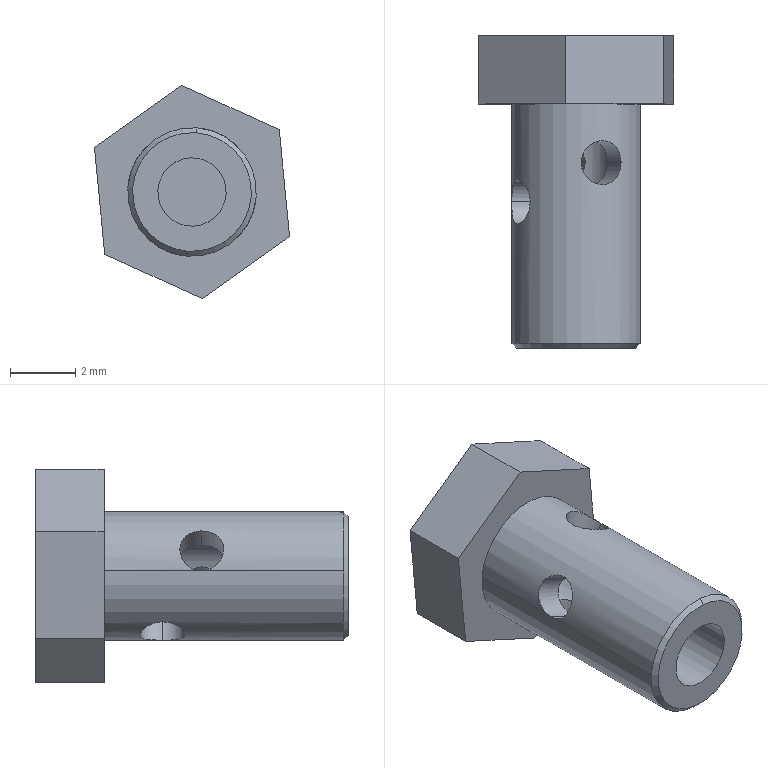Part | STEP file | 2026.6.15-Main Assembly图.sldasm-Part-172 | 1 solid | 24 faces | box 5.989 x 9.6 x 6.551 mm | volume 119.337 mm3 | cylinder 12 | plane 10 | cone 2 | commonest cylinder face diameters 1.35 x8 2.1 x2 3.948 x2
STEP:
#1=CARTESIAN_POINT('',(-1556.242,1444.664,3408.004));
#2=VERTEX_POINT('',#1);
#3=CARTESIAN_POINT('',(-1558.335,1444.664,3408.169));
#4=VERTEX_POINT('',#3);
#5=CARTESIAN_POINT('',(-1557.288,1444.664,3408.086));
#6=DIRECTION('',(0.,-1.,0.));
#7=DIRECTION('',(0.9969,0.,-0.0785));
#8=AXIS2_PLACEMENT_3D('',#5,#6,#7);
#9=CIRCLE('',#8,1.05);
#10=EDGE_CURVE('',#2,#4,#9,.T.);
#11=ORIENTED_EDGE('',*,*,#10,.T.);
#12=CARTESIAN_POINT('',(-1557.288,1444.664,3408.086));
#13=DIRECTION('',(0.,-1.,0.));
#14=DIRECTION('',(0.9969,0.,-0.0785));
#15=AXIS2_PLACEMENT_3D('',#12,#13,#14);
#16=CIRCLE('',#15,1.05);
#17=EDGE_CURVE('',#4,#2,#16,.T.);
#18=ORIENTED_EDGE('',*,*,#17,.T.);
#19=EDGE_LOOP('',(#11,#18));
#20=FACE_OUTER_BOUND('',#19,.T.);
#21=CARTESIAN_POINT('',(-1557.288,1444.664,3408.086));
#22=DIRECTION('',(0.,1.,0.));
#23=DIRECTION('',(1.,0.,0.));
#24=AXIS2_PLACEMENT_3D('',#21,#22,#23);
#25=PLANE('',#24);
#26=ADVANCED_FACE('',(#20),#25,.F.);
#27=CARTESIAN_POINT('',(-1560.283,1446.764,3409.451));
#28=VERTEX_POINT('',#27);
#29=CARTESIAN_POINT('',(-1559.967,1446.764,3406.175));
#30=VERTEX_POINT('',#29);
#31=CARTESIAN_POINT('',(-1559.967,1446.764,3406.175));
#32=DIRECTION('',(0.09585,0.,-0.9954));
#33=VECTOR('',#32,1000.);
#34=LINE('',#31,#33);
#35=EDGE_CURVE('',#28,#30,#34,.T.);
#36=ORIENTED_EDGE('',*,*,#35,.F.);
#37=CARTESIAN_POINT('',(-1557.604,1446.764,3411.362));
#38=VERTEX_POINT('',#37);
#39=CARTESIAN_POINT('',(-1560.283,1446.764,3409.451));
#40=DIRECTION('',(-0.8141,0.,-0.5807));
#41=VECTOR('',#40,1000.);
#42=LINE('',#39,#41);
#43=EDGE_CURVE('',#38,#28,#42,.T.);
#44=ORIENTED_EDGE('',*,*,#43,.F.);
#45=CARTESIAN_POINT('',(-1554.609,1446.764,3409.997));
#46=VERTEX_POINT('',#45);
#47=CARTESIAN_POINT('',(-1557.604,1446.764,3411.362));
#48=DIRECTION('',(-0.91,0.,0.4147));
#49=VECTOR('',#48,1000.);
#50=LINE('',#47,#49);
#51=EDGE_CURVE('',#46,#38,#50,.T.);
#52=ORIENTED_EDGE('',*,*,#51,.F.);
#53=CARTESIAN_POINT('',(-1554.294,1446.764,3406.722));
#54=VERTEX_POINT('',#53);
#55=CARTESIAN_POINT('',(-1554.609,1446.764,3409.997));
#56=DIRECTION('',(-0.09585,0.,0.9954));
#57=VECTOR('',#56,1000.);
#58=LINE('',#55,#57);
#59=EDGE_CURVE('',#54,#46,#58,.T.);
#60=ORIENTED_EDGE('',*,*,#59,.F.);
#61=CARTESIAN_POINT('',(-1556.973,1446.764,3404.811));
#62=VERTEX_POINT('',#61);
#63=CARTESIAN_POINT('',(-1556.973,1446.764,3404.811));
#64=DIRECTION('',(0.8141,0.,0.5807));
#65=VECTOR('',#64,1000.);
#66=LINE('',#63,#65);
#67=EDGE_CURVE('',#62,#54,#66,.T.);
#68=ORIENTED_EDGE('',*,*,#67,.F.);
#69=CARTESIAN_POINT('',(-1559.967,1446.764,3406.175));
#70=DIRECTION('',(0.91,0.,-0.4147));
#71=VECTOR('',#70,1000.);
#72=LINE('',#69,#71);
#73=EDGE_CURVE('',#30,#62,#72,.T.);
#74=ORIENTED_EDGE('',*,*,#73,.F.);
#75=EDGE_LOOP('',(#36,#44,#52,#60,#68,#74));
#76=FACE_OUTER_BOUND('',#75,.T.);
#77=CARTESIAN_POINT('',(-1560.283,1446.764,3409.451));
#78=DIRECTION('',(0.,-1.,0.));
#79=DIRECTION('',(0.,0.,-1.));
#80=AXIS2_PLACEMENT_3D('',#77,#78,#79);
#81=PLANE('',#80);
#82=ADVANCED_FACE('',(#76),#81,.F.);
#83=CARTESIAN_POINT('',(-1558.335,1437.164,3408.169));
#84=VERTEX_POINT('',#83);
#85=CARTESIAN_POINT('',(-1558.335,1441.093,3408.169));
#86=VERTEX_POINT('',#85);
#87=CARTESIAN_POINT('',(-1558.335,1444.664,3408.169));
#88=DIRECTION('',(0.,1.,0.));
#89=VECTOR('',#88,1000.);
#90=LINE('',#87,#89);
#91=EDGE_CURVE('',#84,#86,#90,.T.);
#92=ORIENTED_EDGE('',*,*,#91,.F.);
#93=CARTESIAN_POINT('',(-1556.242,1437.164,3408.004));
#94=VERTEX_POINT('',#93);
#95=CARTESIAN_POINT('',(-1557.288,1437.164,3408.086));
#96=DIRECTION('',(0.,1.,0.));
#97=DIRECTION('',(0.9969,0.,-0.0785));
#98=AXIS2_PLACEMENT_3D('',#95,#96,#97);
#99=CIRCLE('',#98,1.05);
#100=EDGE_CURVE('',#94,#84,#99,.T.);
#101=ORIENTED_EDGE('',*,*,#100,.F.);
#102=CARTESIAN_POINT('',(-1556.242,1441.093,3408.004));
#103=VERTEX_POINT('',#102);
#104=CARTESIAN_POINT('',(-1556.242,1444.664,3408.004));
#105=DIRECTION('',(0.,1.,0.));
#106=VECTOR('',#105,1000.);
#107=LINE('',#104,#106);
#108=EDGE_CURVE('',#94,#103,#107,.T.);
#109=ORIENTED_EDGE('',*,*,#108,.T.);
#110=CARTESIAN_POINT('',(-1556.836,1441.664,3407.139));
#111=VERTEX_POINT('',#110);
#112=CARTESIAN_POINT('',(-1556.242,1441.093,3408.004));
#113=CARTESIAN_POINT('',(-1556.25,1441.03,3407.897));
#114=CARTESIAN_POINT('',(-1556.277,1440.992,3407.778));
#115=CARTESIAN_POINT('',(-1556.376,1440.987,3407.553));
#116=CARTESIAN_POINT('',(-1556.447,1441.019,3407.449));
#117=CARTESIAN_POINT('',(-1556.595,1441.136,3407.291));
#118=CARTESIAN_POINT('',(-1556.673,1441.22,3407.233));
#119=CARTESIAN_POINT('',(-1556.793,1441.42,3407.158));
#120=CARTESIAN_POINT('',(-1556.836,1441.539,3407.139));
#121=CARTESIAN_POINT('',(-1556.836,1441.664,3407.139));
#122=B_SPLINE_CURVE_WITH_KNOTS('',3,(#112,#113,#114,#115,#116,#117,#118,#119,#120,#121),.UNSPECIFIED.,.F.,.F.,(4,2,2,2,4),(0.,0.0003684,0.0007369,0.001105,0.001474),.UNSPECIFIED.);
#123=EDGE_CURVE('',#103,#111,#122,.T.);
#124=ORIENTED_EDGE('',*,*,#123,.T.);
#125=CARTESIAN_POINT('',(-1556.242,1442.236,3408.004));
#126=VERTEX_POINT('',#125);
#127=CARTESIAN_POINT('',(-1556.836,1441.664,3407.139));
#128=CARTESIAN_POINT('',(-1556.836,1441.789,3407.139));
#129=CARTESIAN_POINT('',(-1556.794,1441.908,3407.157));
#130=CARTESIAN_POINT('',(-1556.672,1442.109,3407.233));
#131=CARTESIAN_POINT('',(-1556.594,1442.193,3407.291));
#132=CARTESIAN_POINT('',(-1556.447,1442.309,3407.448));
#133=CARTESIAN_POINT('',(-1556.377,1442.342,3407.55));
#134=CARTESIAN_POINT('',(-1556.277,1442.337,3407.778));
#135=CARTESIAN_POINT('',(-1556.25,1442.299,3407.897));
#136=CARTESIAN_POINT('',(-1556.242,1442.236,3408.004));
#137=B_SPLINE_CURVE_WITH_KNOTS('',3,(#127,#128,#129,#130,#131,#132,#133,#134,#135,#136),.UNSPECIFIED.,.F.,.F.,(4,2,2,2,4),(0.,0.0003676,0.0007352,0.001103,0.00147),.UNSPECIFIED.);
#138=EDGE_CURVE('',#111,#126,#137,.T.);
#139=ORIENTED_EDGE('',*,*,#138,.T.);
#140=CARTESIAN_POINT('',(-1556.242,1444.664,3408.004));
#141=DIRECTION('',(0.,1.,0.));
#142=VECTOR('',#141,1000.);
#143=LINE('',#140,#142);
#144=EDGE_CURVE('',#126,#2,#143,.T.);
#145=ORIENTED_EDGE('',*,*,#144,.T.);
#146=ORIENTED_EDGE('',*,*,#17,.F.);
#147=CARTESIAN_POINT('',(-1558.335,1442.236,3408.169));
#148=VERTEX_POINT('',#147);
#149=CARTESIAN_POINT('',(-1558.335,1444.664,3408.169));
#150=DIRECTION('',(0.,1.,0.));
#151=VECTOR('',#150,1000.);
#152=LINE('',#149,#151);
#153=EDGE_CURVE('',#148,#4,#152,.T.);
#154=ORIENTED_EDGE('',*,*,#153,.F.);
#155=CARTESIAN_POINT('',(-1558.3,1441.664,3407.806));
#156=VERTEX_POINT('',#155);
#157=CARTESIAN_POINT('',(-1558.335,1442.236,3408.169));
#158=CARTESIAN_POINT('',(-1558.343,1442.175,3408.066));
#159=CARTESIAN_POINT('',(-1558.335,1442.093,3407.977));
#160=CARTESIAN_POINT('',(-1558.313,1441.899,3407.847));
#161=CARTESIAN_POINT('',(-1558.3,1441.784,3407.806));
#162=CARTESIAN_POINT('',(-1558.3,1441.664,3407.806));
#163=B_SPLINE_CURVE_WITH_KNOTS('',3,(#157,#158,#159,#160,#161,#162),.UNSPECIFIED.,.F.,.F.,(4,2,4),(0.,0.0003529,0.0007058),.UNSPECIFIED.);
#164=EDGE_CURVE('',#148,#156,#163,.T.);
#165=ORIENTED_EDGE('',*,*,#164,.T.);
#166=CARTESIAN_POINT('',(-1558.3,1441.664,3407.806));
#167=CARTESIAN_POINT('',(-1558.3,1441.545,3407.806));
#168=CARTESIAN_POINT('',(-1558.313,1441.431,3407.846));
#169=CARTESIAN_POINT('',(-1558.335,1441.235,3407.978));
#170=CARTESIAN_POINT('',(-1558.343,1441.153,3408.067));
#171=CARTESIAN_POINT('',(-1558.335,1441.093,3408.169));
#172=B_SPLINE_CURVE_WITH_KNOTS('',3,(#166,#167,#168,#169,#170,#171),.UNSPECIFIED.,.F.,.F.,(4,2,4),(0.,0.0003519,0.0007038),.UNSPECIFIED.);
#173=EDGE_CURVE('',#156,#86,#172,.T.);
#174=ORIENTED_EDGE('',*,*,#173,.T.);
#175=EDGE_LOOP('',(#92,#101,#109,#124,#139,#145,#146,#154,#165,#174));
#176=FACE_OUTER_BOUND('',#175,.T.);
#177=CARTESIAN_POINT('',(-1558.236,1442.864,3407.634));
#178=VERTEX_POINT('',#177);
#179=CARTESIAN_POINT('',(-1557.008,1442.864,3407.075));
#180=VERTEX_POINT('',#179);
#181=CARTESIAN_POINT('',(-1558.236,1442.864,3407.634));
#182=CARTESIAN_POINT('',(-1558.236,1443.049,3407.634));
#183=CARTESIAN_POINT('',(-1558.196,1443.219,3407.541));
#184=CARTESIAN_POINT('',(-1558.069,1443.401,3407.381));
#185=CARTESIAN_POINT('',(-1558.015,1443.451,3407.324));
#186=CARTESIAN_POINT('',(-1557.885,1443.52,3407.218));
#187=CARTESIAN_POINT('',(-1557.808,1443.539,3407.17));
#188=CARTESIAN_POINT('',(-1557.641,1443.539,3407.093));
#189=CARTESIAN_POINT('',(-1557.553,1443.52,3407.067));
#190=CARTESIAN_POINT('',(-1557.387,1443.451,3407.038));
#191=CARTESIAN_POINT('',(-1557.308,1443.401,3407.034));
#192=CARTESIAN_POINT('',(-1557.105,1443.219,3407.044));
#193=CARTESIAN_POINT('',(-1557.008,1443.049,3407.075));
#194=CARTESIAN_POINT('',(-1557.008,1442.864,3407.075));
#195=B_SPLINE_CURVE_WITH_KNOTS('',3,(#181,#182,#183,#184,#185,#186,#187,#188,#189,#190,#191,#192,#193,#194),.UNSPECIFIED.,.F.,.F.,(4,2,2,2,2,2,4),(0.,0.0005437,0.0008156,0.001087,0.001359,0.001631,0.002175),.UNSPECIFIED.);
#196=EDGE_CURVE('',#178,#180,#195,.T.);
#197=ORIENTED_EDGE('',*,*,#196,.T.);
#198=CARTESIAN_POINT('',(-1557.008,1442.864,3407.075));
#199=CARTESIAN_POINT('',(-1557.008,1442.68,3407.075));
#200=CARTESIAN_POINT('',(-1557.105,1442.51,3407.044));
#201=CARTESIAN_POINT('',(-1557.308,1442.328,3407.034));
#202=CARTESIAN_POINT('',(-1557.386,1442.278,3407.038));
#203=CARTESIAN_POINT('',(-1557.552,1442.209,3407.067));
#204=CARTESIAN_POINT('',(-1557.639,1442.189,3407.092));
#205=CARTESIAN_POINT('',(-1557.806,1442.189,3407.168));
#206=CARTESIAN_POINT('',(-1557.884,1442.208,3407.217));
#207=CARTESIAN_POINT('',(-1558.015,1442.277,3407.324));
#208=CARTESIAN_POINT('',(-1558.069,1442.327,3407.381));
#209=CARTESIAN_POINT('',(-1558.196,1442.51,3407.541));
#210=CARTESIAN_POINT('',(-1558.236,1442.679,3407.634));
#211=CARTESIAN_POINT('',(-1558.236,1442.864,3407.634));
#212=B_SPLINE_CURVE_WITH_KNOTS('',3,(#198,#199,#200,#201,#202,#203,#204,#205,#206,#207,#208,#209,#210,#211),.UNSPECIFIED.,.F.,.F.,(4,2,2,2,2,2,4),(0.,0.0005437,0.0008156,0.001087,0.001359,0.001631,0.002175),.UNSPECIFIED.);
#213=EDGE_CURVE('',#180,#178,#212,.T.);
#214=ORIENTED_EDGE('',*,*,#213,.T.);
#215=EDGE_LOOP('',(#197,#214));
#216=FACE_BOUND('',#215,.T.);
#217=CARTESIAN_POINT('',(-1557.288,1444.664,3408.086));
#218=DIRECTION('',(0.,1.,0.));
#219=DIRECTION('',(-0.9969,0.,0.0785));
#220=AXIS2_PLACEMENT_3D('',#217,#218,#219);
#221=CYLINDRICAL_SURFACE('',#220,1.05);
#222=ADVANCED_FACE('',(#176,#216),#221,.F.);
#223=CARTESIAN_POINT('',(-1557.604,1444.664,3411.362));
#224=VERTEX_POINT('',#223);
#225=CARTESIAN_POINT('',(-1557.604,1437.164,3411.362));
#226=DIRECTION('',(0.,1.,0.));
#227=VECTOR('',#226,1000.);
#228=LINE('',#225,#227);
#229=EDGE_CURVE('',#224,#38,#228,.T.);
#230=ORIENTED_EDGE('',*,*,#229,.F.);
#231=CARTESIAN_POINT('',(-1554.609,1444.664,3409.997));
#232=VERTEX_POINT('',#231);
#233=CARTESIAN_POINT('',(-1554.609,1444.664,3409.997));
#234=DIRECTION('',(-0.91,0.,0.4147));
#235=VECTOR('',#234,1000.);
#236=LINE('',#233,#235);
#237=EDGE_CURVE('',#232,#224,#236,.T.);
#238=ORIENTED_EDGE('',*,*,#237,.F.);
#239=CARTESIAN_POINT('',(-1554.609,1437.164,3409.997));
#240=DIRECTION('',(0.,-1.,0.));
#241=VECTOR('',#240,1000.);
#242=LINE('',#239,#241);
#243=EDGE_CURVE('',#46,#232,#242,.T.);
#244=ORIENTED_EDGE('',*,*,#243,.F.);
#245=ORIENTED_EDGE('',*,*,#51,.T.);
#246=EDGE_LOOP('',(#230,#238,#244,#245));
#247=FACE_OUTER_BOUND('',#246,.T.);
#248=CARTESIAN_POINT('',(-1557.604,1437.164,3411.362));
#249=DIRECTION('',(0.4147,0.,0.91));
#250=DIRECTION('',(-0.91,0.,0.4147));
#251=AXIS2_PLACEMENT_3D('',#248,#249,#250);
#252=PLANE('',#251);
#253=ADVANCED_FACE('',(#247),#252,.T.);
#254=CARTESIAN_POINT('',(-1560.283,1444.664,3409.451));
#255=VERTEX_POINT('',#254);
#256=CARTESIAN_POINT('',(-1560.283,1437.164,3409.451));
#257=DIRECTION('',(0.,1.,0.));
#258=VECTOR('',#257,1000.);
#259=LINE('',#256,#258);
#260=EDGE_CURVE('',#255,#28,#259,.T.);
#261=ORIENTED_EDGE('',*,*,#260,.F.);
#262=CARTESIAN_POINT('',(-1557.604,1444.664,3411.362));
#263=DIRECTION('',(-0.8141,0.,-0.5807));
#264=VECTOR('',#263,1000.);
#265=LINE('',#262,#264);
#266=EDGE_CURVE('',#224,#255,#265,.T.);
#267=ORIENTED_EDGE('',*,*,#266,.F.);
#268=ORIENTED_EDGE('',*,*,#229,.T.);
#269=ORIENTED_EDGE('',*,*,#43,.T.);
#270=EDGE_LOOP('',(#261,#267,#268,#269));
#271=FACE_OUTER_BOUND('',#270,.T.);
#272=CARTESIAN_POINT('',(-1560.283,1437.164,3409.451));
#273=DIRECTION('',(-0.5807,0.,0.8141));
#274=DIRECTION('',(0.,1.,0.));
#275=AXIS2_PLACEMENT_3D('',#272,#273,#274);
#276=PLANE('',#275);
#277=ADVANCED_FACE('',(#271),#276,.T.);
#278=CARTESIAN_POINT('',(-1559.967,1444.664,3406.175));
#279=VERTEX_POINT('',#278);
#280=CARTESIAN_POINT('',(-1559.967,1437.164,3406.175));
#281=DIRECTION('',(0.,1.,0.));
#282=VECTOR('',#281,1000.);
#283=LINE('',#280,#282);
#284=EDGE_CURVE('',#279,#30,#283,.T.);
#285=ORIENTED_EDGE('',*,*,#284,.F.);
#286=CARTESIAN_POINT('',(-1560.283,1444.664,3409.451));
#287=DIRECTION('',(0.09585,0.,-0.9954));
#288=VECTOR('',#287,1000.);
#289=LINE('',#286,#288);
#290=EDGE_CURVE('',#255,#279,#289,.T.);
#291=ORIENTED_EDGE('',*,*,#290,.F.);
#292=ORIENTED_EDGE('',*,*,#260,.T.);
#293=ORIENTED_EDGE('',*,*,#35,.T.);
#294=EDGE_LOOP('',(#285,#291,#292,#293));
#295=FACE_OUTER_BOUND('',#294,.T.);
#296=CARTESIAN_POINT('',(-1559.967,1437.164,3406.175));
#297=DIRECTION('',(-0.9954,0.,-0.09585));
#298=DIRECTION('',(0.,1.,0.));
#299=AXIS2_PLACEMENT_3D('',#296,#297,#298);
#300=PLANE('',#299);
#301=ADVANCED_FACE('',(#295),#300,.T.);
#302=CARTESIAN_POINT('',(-1556.973,1444.664,3404.811));
#303=VERTEX_POINT('',#302);
#304=CARTESIAN_POINT('',(-1556.973,1437.164,3404.811));
#305=DIRECTION('',(0.,1.,0.));
#306=VECTOR('',#305,1000.);
#307=LINE('',#304,#306);
#308=EDGE_CURVE('',#303,#62,#307,.T.);
#309=ORIENTED_EDGE('',*,*,#308,.F.);
#310=CARTESIAN_POINT('',(-1559.967,1444.664,3406.175));
#311=DIRECTION('',(0.91,0.,-0.4147));
#312=VECTOR('',#311,1000.);
#313=LINE('',#310,#312);
#314=EDGE_CURVE('',#279,#303,#313,.T.);
#315=ORIENTED_EDGE('',*,*,#314,.F.);
#316=ORIENTED_EDGE('',*,*,#284,.T.);
#317=ORIENTED_EDGE('',*,*,#73,.T.);
#318=EDGE_LOOP('',(#309,#315,#316,#317));
#319=FACE_OUTER_BOUND('',#318,.T.);
#320=CARTESIAN_POINT('',(-1559.967,1437.164,3406.175));
#321=DIRECTION('',(-0.4147,0.,-0.91));
#322=DIRECTION('',(0.,1.,0.));
#323=AXIS2_PLACEMENT_3D('',#320,#321,#322);
#324=PLANE('',#323);
#325=ADVANCED_FACE('',(#319),#324,.T.);
#326=CARTESIAN_POINT('',(-1554.294,1444.664,3406.722));
#327=VERTEX_POINT('',#326);
#328=CARTESIAN_POINT('',(-1554.294,1437.164,3406.722));
#329=DIRECTION('',(0.,1.,0.));
#330=VECTOR('',#329,1000.);
#331=LINE('',#328,#330);
#332=EDGE_CURVE('',#327,#54,#331,.T.);
#333=ORIENTED_EDGE('',*,*,#332,.F.);
#334=CARTESIAN_POINT('',(-1556.973,1444.664,3404.811));
#335=DIRECTION('',(0.8141,0.,0.5807));
#336=VECTOR('',#335,1000.);
#337=LINE('',#334,#336);
#338=EDGE_CURVE('',#303,#327,#337,.T.);
#339=ORIENTED_EDGE('',*,*,#338,.F.);
#340=ORIENTED_EDGE('',*,*,#308,.T.);
#341=ORIENTED_EDGE('',*,*,#67,.T.);
#342=EDGE_LOOP('',(#333,#339,#340,#341));
#343=FACE_OUTER_BOUND('',#342,.T.);
#344=CARTESIAN_POINT('',(-1556.973,1437.164,3404.811));
#345=DIRECTION('',(0.5807,0.,-0.8141));
#346=DIRECTION('',(0.,-1.,0.));
#347=AXIS2_PLACEMENT_3D('',#344,#345,#346);
#348=PLANE('',#347);
#349=ADVANCED_FACE('',(#343),#348,.T.);
#350=ORIENTED_EDGE('',*,*,#243,.T.);
#351=CARTESIAN_POINT('',(-1554.294,1444.664,3406.722));
#352=DIRECTION('',(-0.09585,0.,0.9954));
#353=VECTOR('',#352,1000.);
#354=LINE('',#351,#353);
#355=EDGE_CURVE('',#327,#232,#354,.T.);
#356=ORIENTED_EDGE('',*,*,#355,.F.);
#357=ORIENTED_EDGE('',*,*,#332,.T.);
#358=ORIENTED_EDGE('',*,*,#59,.T.);
#359=EDGE_LOOP('',(#350,#356,#357,#358));
#360=FACE_OUTER_BOUND('',#359,.T.);
#361=CARTESIAN_POINT('',(-1554.609,1437.164,3409.997));
#362=DIRECTION('',(0.9954,0.,0.09585));
#363=DIRECTION('',(-0.09585,0.,0.9954));
#364=AXIS2_PLACEMENT_3D('',#361,#362,#363);
#365=PLANE('',#364);
#366=ADVANCED_FACE('',(#360),#365,.T.);
#367=CARTESIAN_POINT('',(-1559.256,1441.664,3408.241));
#368=VERTEX_POINT('',#367);
#369=CARTESIAN_POINT('',(-1569.362,1441.664,3412.847));
#370=DIRECTION('',(0.91,0.,-0.4147));
#371=VECTOR('',#370,1000.);
#372=LINE('',#369,#371);
#373=EDGE_CURVE('',#368,#156,#372,.T.);
#374=ORIENTED_EDGE('',*,*,#373,.T.);
#375=ORIENTED_EDGE('',*,*,#164,.F.);
#376=CARTESIAN_POINT('',(-1557.74,1441.664,3409.034));
#377=VERTEX_POINT('',#376);
#378=CARTESIAN_POINT('',(-1557.74,1441.664,3409.034));
#379=CARTESIAN_POINT('',(-1557.74,1441.789,3409.034));
#380=CARTESIAN_POINT('',(-1557.783,1441.908,3409.015));
#381=CARTESIAN_POINT('',(-1557.905,1442.109,3408.939));
#382=CARTESIAN_POINT('',(-1557.982,1442.193,3408.882));
#383=CARTESIAN_POINT('',(-1558.129,1442.309,3408.724));
#384=CARTESIAN_POINT('',(-1558.199,1442.342,3408.623));
#385=CARTESIAN_POINT('',(-1558.3,1442.337,3408.395));
#386=CARTESIAN_POINT('',(-1558.327,1442.299,3408.276));
#387=CARTESIAN_POINT('',(-1558.335,1442.236,3408.169));
#388=B_SPLINE_CURVE_WITH_KNOTS('',3,(#378,#379,#380,#381,#382,#383,#384,#385,#386,#387),.UNSPECIFIED.,.F.,.F.,(4,2,2,2,4),(0.,0.0003676,0.0007352,0.001103,0.00147),.UNSPECIFIED.);
#389=EDGE_CURVE('',#377,#148,#388,.T.);
#390=ORIENTED_EDGE('',*,*,#389,.F.);
#391=CARTESIAN_POINT('',(-1558.696,1441.664,3409.47));
#392=VERTEX_POINT('',#391);
#393=CARTESIAN_POINT('',(-1568.802,1441.664,3414.075));
#394=DIRECTION('',(0.91,0.,-0.4147));
#395=VECTOR('',#394,1000.);
#396=LINE('',#393,#395);
#397=EDGE_CURVE('',#392,#377,#396,.T.);
#398=ORIENTED_EDGE('',*,*,#397,.F.);
#399=CARTESIAN_POINT('',(-1559.256,1441.664,3408.241));
#400=CARTESIAN_POINT('',(-1559.256,1441.754,3408.241));
#401=CARTESIAN_POINT('',(-1559.255,1441.842,3408.261));
#402=CARTESIAN_POINT('',(-1559.247,1442.005,3408.332));
#403=CARTESIAN_POINT('',(-1559.241,1442.08,3408.384));
#404=CARTESIAN_POINT('',(-1559.218,1442.203,3408.509));
#405=CARTESIAN_POINT('',(-1559.2,1442.253,3408.583));
#406=CARTESIAN_POINT('',(-1559.153,1442.321,3408.74));
#407=CARTESIAN_POINT('',(-1559.122,1442.339,3408.823));
#408=CARTESIAN_POINT('',(-1559.048,1442.339,3408.985));
#409=CARTESIAN_POINT('',(-1559.006,1442.322,3409.063));
#410=CARTESIAN_POINT('',(-1558.918,1442.254,3409.204));
#411=CARTESIAN_POINT('',(-1558.873,1442.204,3409.265));
#412=CARTESIAN_POINT('',(-1558.754,1442.018,3409.415));
#413=CARTESIAN_POINT('',(-1558.696,1441.844,3409.47));
#414=CARTESIAN_POINT('',(-1558.696,1441.664,3409.47));
#415=B_SPLINE_CURVE_WITH_KNOTS('',3,(#399,#400,#401,#402,#403,#404,#405,#406,#407,#408,#409,#410,#411,#412,#413,#414),.UNSPECIFIED.,.F.,.F.,(4,2,2,2,2,2,2,4),(0.,0.0002657,0.0005314,0.0007971,0.001063,0.001329,0.001594,0.002126),.UNSPECIFIED.);
#416=EDGE_CURVE('',#368,#392,#415,.T.);
#417=ORIENTED_EDGE('',*,*,#416,.F.);
#418=EDGE_LOOP('',(#374,#375,#390,#398,#417));
#419=FACE_OUTER_BOUND('',#418,.T.);
#420=CARTESIAN_POINT('',(-1569.082,1441.664,3413.461));
#421=DIRECTION('',(-0.91,0.,0.4147));
#422=DIRECTION('',(-0.4147,0.,-0.91));
#423=AXIS2_PLACEMENT_3D('',#420,#421,#422);
#424=CYLINDRICAL_SURFACE('',#423,0.675);
#425=ADVANCED_FACE('',(#419),#424,.F.);
#426=CARTESIAN_POINT('',(-1557.569,1442.864,3409.098));
#427=VERTEX_POINT('',#426);
#428=CARTESIAN_POINT('',(-1557.133,1442.864,3410.054));
#429=VERTEX_POINT('',#428);
#430=CARTESIAN_POINT('',(-1552.528,1442.864,3420.16));
#431=DIRECTION('',(0.4147,0.,0.91));
#432=VECTOR('',#431,1000.);
#433=LINE('',#430,#432);
#434=EDGE_CURVE('',#427,#429,#433,.T.);
#435=ORIENTED_EDGE('',*,*,#434,.F.);
#436=CARTESIAN_POINT('',(-1556.341,1442.864,3408.538));
#437=VERTEX_POINT('',#436);
#438=CARTESIAN_POINT('',(-1556.341,1442.864,3408.538));
#439=CARTESIAN_POINT('',(-1556.341,1443.049,3408.538));
#440=CARTESIAN_POINT('',(-1556.381,1443.219,3408.632));
#441=CARTESIAN_POINT('',(-1556.507,1443.401,3408.792));
#442=CARTESIAN_POINT('',(-1556.561,1443.451,3408.848));
#443=CARTESIAN_POINT('',(-1556.692,1443.52,3408.954));
#444=CARTESIAN_POINT('',(-1556.768,1443.539,3409.003));
#445=CARTESIAN_POINT('',(-1556.935,1443.539,3409.079));
#446=CARTESIAN_POINT('',(-1557.023,1443.52,3409.106));
#447=CARTESIAN_POINT('',(-1557.189,1443.451,3409.135));
#448=CARTESIAN_POINT('',(-1557.268,1443.401,3409.138));
#449=CARTESIAN_POINT('',(-1557.472,1443.219,3409.129));
#450=CARTESIAN_POINT('',(-1557.569,1443.049,3409.098));
#451=CARTESIAN_POINT('',(-1557.569,1442.864,3409.098));
#452=B_SPLINE_CURVE_WITH_KNOTS('',3,(#438,#439,#440,#441,#442,#443,#444,#445,#446,#447,#448,#449,#450,#451),.UNSPECIFIED.,.F.,.F.,(4,2,2,2,2,2,4),(0.,0.0005437,0.0008156,0.001087,0.001359,0.001631,0.002175),.UNSPECIFIED.);
#453=EDGE_CURVE('',#437,#427,#452,.T.);
#454=ORIENTED_EDGE('',*,*,#453,.F.);
#455=CARTESIAN_POINT('',(-1555.905,1442.864,3409.494));
#456=VERTEX_POINT('',#455);
#457=CARTESIAN_POINT('',(-1551.299,1442.864,3419.6));
#458=DIRECTION('',(0.4147,0.,0.91));
#459=VECTOR('',#458,1000.);
#460=LINE('',#457,#459);
#461=EDGE_CURVE('',#437,#456,#460,.T.);
#462=ORIENTED_EDGE('',*,*,#461,.T.);
#463=CARTESIAN_POINT('',(-1557.133,1442.864,3410.054));
#464=CARTESIAN_POINT('',(-1557.133,1442.954,3410.054));
#465=CARTESIAN_POINT('',(-1557.114,1443.042,3410.053));
#466=CARTESIAN_POINT('',(-1557.043,1443.205,3410.045));
#467=CARTESIAN_POINT('',(-1556.991,1443.28,3410.039));
#468=CARTESIAN_POINT('',(-1556.866,1443.403,3410.016));
#469=CARTESIAN_POINT('',(-1556.791,1443.453,3409.999));
#470=CARTESIAN_POINT('',(-1556.635,1443.521,3409.951));
#471=CARTESIAN_POINT('',(-1556.551,1443.539,3409.92));
#472=CARTESIAN_POINT('',(-1556.39,1443.539,3409.846));
#473=CARTESIAN_POINT('',(-1556.311,1443.522,3409.804));
#474=CARTESIAN_POINT('',(-1556.171,1443.454,3409.716));
#475=CARTESIAN_POINT('',(-1556.11,1443.404,3409.671));
#476=CARTESIAN_POINT('',(-1555.96,1443.218,3409.552));
#477=CARTESIAN_POINT('',(-1555.905,1443.044,3409.494));
#478=CARTESIAN_POINT('',(-1555.905,1442.864,3409.494));
#479=B_SPLINE_CURVE_WITH_KNOTS('',3,(#463,#464,#465,#466,#467,#468,#469,#470,#471,#472,#473,#474,#475,#476,#477,#478),.UNSPECIFIED.,.F.,.F.,(4,2,2,2,2,2,2,4),(0.,0.0002657,0.0005314,0.0007971,0.001063,0.001329,0.001594,0.002126),.UNSPECIFIED.);
#480=EDGE_CURVE('',#429,#456,#479,.T.);
#481=ORIENTED_EDGE('',*,*,#480,.F.);
#482=EDGE_LOOP('',(#435,#454,#462,#481));
#483=FACE_OUTER_BOUND('',#482,.T.);
#484=CARTESIAN_POINT('',(-1551.914,1442.864,3419.88));
#485=DIRECTION('',(0.4147,0.,0.91));
#486=DIRECTION('',(-0.91,0.,0.4147));
#487=AXIS2_PLACEMENT_3D('',#484,#485,#486);
#488=CYLINDRICAL_SURFACE('',#487,0.675);
#489=ADVANCED_FACE('',(#483),#488,.F.);
#490=CARTESIAN_POINT('',(-1557.431,1437.164,3406.268));
#491=VERTEX_POINT('',#490);
#492=CARTESIAN_POINT('',(-1557.145,1437.164,3409.905));
#493=VERTEX_POINT('',#492);
#494=CARTESIAN_POINT('',(-1557.288,1437.164,3408.086));
#495=DIRECTION('',(0.,1.,0.));
#496=DIRECTION('',(-0.0785,0.,-0.9969));
#497=AXIS2_PLACEMENT_3D('',#494,#495,#496);
#498=CIRCLE('',#497,1.824);
#499=EDGE_CURVE('',#491,#493,#498,.T.);
#500=ORIENTED_EDGE('',*,*,#499,.F.);
#501=CARTESIAN_POINT('',(-1557.288,1437.164,3408.086));
#502=DIRECTION('',(0.,1.,0.));
#503=DIRECTION('',(-0.0785,0.,-0.9969));
#504=AXIS2_PLACEMENT_3D('',#501,#502,#503);
#505=CIRCLE('',#504,1.824);
#506=EDGE_CURVE('',#493,#491,#505,.T.);
#507=ORIENTED_EDGE('',*,*,#506,.F.);
#508=EDGE_LOOP('',(#500,#507));
#509=FACE_OUTER_BOUND('',#508,.T.);
#510=ORIENTED_EDGE('',*,*,#100,.T.);
#511=CARTESIAN_POINT('',(-1557.288,1437.164,3408.086));
#512=DIRECTION('',(0.,1.,0.));
#513=DIRECTION('',(0.9969,0.,-0.0785));
#514=AXIS2_PLACEMENT_3D('',#511,#512,#513);
#515=CIRCLE('',#514,1.05);
#516=EDGE_CURVE('',#84,#94,#515,.T.);
#517=ORIENTED_EDGE('',*,*,#516,.T.);
#518=EDGE_LOOP('',(#510,#517));
#519=FACE_BOUND('',#518,.T.);
#520=CARTESIAN_POINT('',(-1560.283,1437.164,3409.451));
#521=DIRECTION('',(0.,-1.,0.));
#522=DIRECTION('',(0.,0.,-1.));
#523=AXIS2_PLACEMENT_3D('',#520,#521,#522);
#524=PLANE('',#523);
#525=ADVANCED_FACE('',(#509,#519),#524,.T.);
#526=CARTESIAN_POINT('',(-1557.443,1442.864,3406.118));
#527=VERTEX_POINT('',#526);
#528=CARTESIAN_POINT('',(-1562.049,1442.864,3396.013));
#529=DIRECTION('',(0.4147,0.,0.91));
#530=VECTOR('',#529,1000.);
#531=LINE('',#528,#530);
#532=EDGE_CURVE('',#527,#180,#531,.T.);
#533=ORIENTED_EDGE('',*,*,#532,.T.);
#534=ORIENTED_EDGE('',*,*,#196,.F.);
#535=CARTESIAN_POINT('',(-1558.672,1442.864,3406.678));
#536=VERTEX_POINT('',#535);
#537=CARTESIAN_POINT('',(-1563.277,1442.864,3396.573));
#538=DIRECTION('',(0.4147,0.,0.91));
#539=VECTOR('',#538,1000.);
#540=LINE('',#537,#539);
#541=EDGE_CURVE('',#536,#178,#540,.T.);
#542=ORIENTED_EDGE('',*,*,#541,.F.);
#543=CARTESIAN_POINT('',(-1557.443,1442.864,3406.118));
#544=CARTESIAN_POINT('',(-1557.443,1442.954,3406.118));
#545=CARTESIAN_POINT('',(-1557.462,1443.042,3406.12));
#546=CARTESIAN_POINT('',(-1557.534,1443.205,3406.127));
#547=CARTESIAN_POINT('',(-1557.586,1443.28,3406.134));
#548=CARTESIAN_POINT('',(-1557.711,1443.403,3406.157));
#549=CARTESIAN_POINT('',(-1557.785,1443.453,3406.174));
#550=CARTESIAN_POINT('',(-1557.942,1443.521,3406.222));
#551=CARTESIAN_POINT('',(-1558.025,1443.539,3406.253));
#552=CARTESIAN_POINT('',(-1558.187,1443.539,3406.327));
#553=CARTESIAN_POINT('',(-1558.265,1443.522,3406.369));
#554=CARTESIAN_POINT('',(-1558.406,1443.454,3406.457));
#555=CARTESIAN_POINT('',(-1558.467,1443.404,3406.501));
#556=CARTESIAN_POINT('',(-1558.617,1443.218,3406.621));
#557=CARTESIAN_POINT('',(-1558.672,1443.044,3406.678));
#558=CARTESIAN_POINT('',(-1558.672,1442.864,3406.678));
#559=B_SPLINE_CURVE_WITH_KNOTS('',3,(#543,#544,#545,#546,#547,#548,#549,#550,#551,#552,#553,#554,#555,#556,#557,#558),.UNSPECIFIED.,.F.,.F.,(4,2,2,2,2,2,2,4),(0.,0.0002657,0.0005314,0.0007971,0.001063,0.001329,0.001594,0.002126),.UNSPECIFIED.);
#560=EDGE_CURVE('',#527,#536,#559,.T.);
#561=ORIENTED_EDGE('',*,*,#560,.F.);
#562=EDGE_LOOP('',(#533,#534,#542,#561));
#563=FACE_OUTER_BOUND('',#562,.T.);
#564=CARTESIAN_POINT('',(-1562.663,1442.864,3396.293));
#565=DIRECTION('',(-0.4147,0.,-0.91));
#566=DIRECTION('',(0.91,0.,-0.4147));
#567=AXIS2_PLACEMENT_3D('',#564,#565,#566);
#568=CYLINDRICAL_SURFACE('',#567,0.675);
#569=ADVANCED_FACE('',(#563),#568,.F.);
#570=CARTESIAN_POINT('',(-1556.276,1441.664,3408.367));
#571=VERTEX_POINT('',#570);
#572=CARTESIAN_POINT('',(-1555.32,1441.664,3407.931));
#573=VERTEX_POINT('',#572);
#574=CARTESIAN_POINT('',(-1545.215,1441.664,3403.326));
#575=DIRECTION('',(0.91,0.,-0.4147));
#576=VECTOR('',#575,1000.);
#577=LINE('',#574,#576);
#578=EDGE_CURVE('',#571,#573,#577,.T.);
#579=ORIENTED_EDGE('',*,*,#578,.F.);
#580=CARTESIAN_POINT('',(-1556.242,1442.236,3408.004));
#581=CARTESIAN_POINT('',(-1556.233,1442.175,3408.106));
#582=CARTESIAN_POINT('',(-1556.242,1442.093,3408.195));
#583=CARTESIAN_POINT('',(-1556.264,1441.899,3408.326));
#584=CARTESIAN_POINT('',(-1556.276,1441.784,3408.367));
#585=CARTESIAN_POINT('',(-1556.276,1441.664,3408.367));
#586=B_SPLINE_CURVE_WITH_KNOTS('',3,(#580,#581,#582,#583,#584,#585),.UNSPECIFIED.,.F.,.F.,(4,2,4),(0.,0.0003529,0.0007058),.UNSPECIFIED.);
#587=EDGE_CURVE('',#126,#571,#586,.T.);
#588=ORIENTED_EDGE('',*,*,#587,.F.);
#589=ORIENTED_EDGE('',*,*,#138,.F.);
#590=CARTESIAN_POINT('',(-1555.88,1441.664,3406.703));
#591=VERTEX_POINT('',#590);
#592=CARTESIAN_POINT('',(-1545.775,1441.664,3402.098));
#593=DIRECTION('',(0.91,0.,-0.4147));
#594=VECTOR('',#593,1000.);
#595=LINE('',#592,#594);
#596=EDGE_CURVE('',#111,#591,#595,.T.);
#597=ORIENTED_EDGE('',*,*,#596,.T.);
#598=CARTESIAN_POINT('',(-1555.32,1441.664,3407.931));
#599=CARTESIAN_POINT('',(-1555.32,1441.754,3407.931));
#600=CARTESIAN_POINT('',(-1555.322,1441.842,3407.912));
#601=CARTESIAN_POINT('',(-1555.329,1442.005,3407.841));
#602=CARTESIAN_POINT('',(-1555.336,1442.08,3407.789));
#603=CARTESIAN_POINT('',(-1555.359,1442.203,3407.664));
#604=CARTESIAN_POINT('',(-1555.376,1442.253,3407.59));
#605=CARTESIAN_POINT('',(-1555.424,1442.321,3407.433));
#606=CARTESIAN_POINT('',(-1555.455,1442.339,3407.349));
#607=CARTESIAN_POINT('',(-1555.528,1442.339,3407.188));
#608=CARTESIAN_POINT('',(-1555.571,1442.322,3407.109));
#609=CARTESIAN_POINT('',(-1555.659,1442.254,3406.969));
#610=CARTESIAN_POINT('',(-1555.703,1442.204,3406.908));
#611=CARTESIAN_POINT('',(-1555.823,1442.018,3406.758));
#612=CARTESIAN_POINT('',(-1555.88,1441.844,3406.703));
#613=CARTESIAN_POINT('',(-1555.88,1441.664,3406.703));
#614=B_SPLINE_CURVE_WITH_KNOTS('',3,(#598,#599,#600,#601,#602,#603,#604,#605,#606,#607,#608,#609,#610,#611,#612,#613),.UNSPECIFIED.,.F.,.F.,(4,2,2,2,2,2,2,4),(0.,0.0002657,0.0005314,0.0007971,0.001063,0.001329,0.001594,0.002126),.UNSPECIFIED.);
#615=EDGE_CURVE('',#573,#591,#614,.T.);
#616=ORIENTED_EDGE('',*,*,#615,.F.);
#617=EDGE_LOOP('',(#579,#588,#589,#597,#616));
#618=FACE_OUTER_BOUND('',#617,.T.);
#619=CARTESIAN_POINT('',(-1545.495,1441.664,3402.712));
#620=DIRECTION('',(0.91,0.,-0.4147));
#621=DIRECTION('',(0.4147,0.,0.91));
#622=AXIS2_PLACEMENT_3D('',#619,#620,#621);
#623=CYLINDRICAL_SURFACE('',#622,0.675);
#624=ADVANCED_FACE('',(#618),#623,.F.);
#625=ORIENTED_EDGE('',*,*,#338,.T.);
#626=ORIENTED_EDGE('',*,*,#355,.T.);
#627=ORIENTED_EDGE('',*,*,#237,.T.);
#628=ORIENTED_EDGE('',*,*,#266,.T.);
#629=ORIENTED_EDGE('',*,*,#290,.T.);
#630=ORIENTED_EDGE('',*,*,#314,.T.);
#631=EDGE_LOOP('',(#625,#626,#627,#628,#629,#630));
#632=FACE_OUTER_BOUND('',#631,.T.);
#633=CARTESIAN_POINT('',(-1555.32,1444.664,3407.931));
#634=VERTEX_POINT('',#633);
#635=CARTESIAN_POINT('',(-1559.256,1444.664,3408.241));
#636=VERTEX_POINT('',#635);
#637=CARTESIAN_POINT('',(-1557.288,1444.664,3408.086));
#638=DIRECTION('',(0.,-1.,0.));
#639=DIRECTION('',(0.9969,0.,-0.0785));
#640=AXIS2_PLACEMENT_3D('',#637,#638,#639);
#641=CIRCLE('',#640,1.974);
#642=EDGE_CURVE('',#634,#636,#641,.T.);
#643=ORIENTED_EDGE('',*,*,#642,.F.);
#644=CARTESIAN_POINT('',(-1557.288,1444.664,3408.086));
#645=DIRECTION('',(0.,-1.,0.));
#646=DIRECTION('',(0.9969,0.,-0.0785));
#647=AXIS2_PLACEMENT_3D('',#644,#645,#646);
#648=CIRCLE('',#647,1.974);
#649=EDGE_CURVE('',#636,#634,#648,.T.);
#650=ORIENTED_EDGE('',*,*,#649,.F.);
#651=EDGE_LOOP('',(#643,#650));
#652=FACE_BOUND('',#651,.T.);
#653=CARTESIAN_POINT('',(-1556.882,1444.664,3408.983));
#654=DIRECTION('',(0.,-1.,0.));
#655=DIRECTION('',(0.,0.,-1.));
#656=AXIS2_PLACEMENT_3D('',#653,#654,#655);
#657=PLANE('',#656);
#658=ADVANCED_FACE('',(#632,#652),#657,.T.);
#659=CARTESIAN_POINT('',(-1557.133,1437.314,3410.054));
#660=VERTEX_POINT('',#659);
#661=CARTESIAN_POINT('',(-1557.133,1437.314,3410.054));
#662=DIRECTION('',(0.0555,0.7071,0.7049));
#663=VECTOR('',#662,1000.);
#664=LINE('',#661,#663);
#665=EDGE_CURVE('',#493,#660,#664,.T.);
#666=ORIENTED_EDGE('',*,*,#665,.F.);
#667=ORIENTED_EDGE('',*,*,#506,.T.);
#668=CARTESIAN_POINT('',(-1557.443,1437.314,3406.118));
#669=VERTEX_POINT('',#668);
#670=CARTESIAN_POINT('',(-1557.443,1437.314,3406.118));
#671=DIRECTION('',(-0.0555,0.7071,-0.7049));
#672=VECTOR('',#671,1000.);
#673=LINE('',#670,#672);
#674=EDGE_CURVE('',#491,#669,#673,.T.);
#675=ORIENTED_EDGE('',*,*,#674,.T.);
#676=CARTESIAN_POINT('',(-1555.32,1437.314,3407.931));
#677=VERTEX_POINT('',#676);
#678=CARTESIAN_POINT('',(-1557.288,1437.314,3408.086));
#679=DIRECTION('',(0.,1.,0.));
#680=DIRECTION('',(0.9969,0.,-0.0785));
#681=AXIS2_PLACEMENT_3D('',#678,#679,#680);
#682=CIRCLE('',#681,1.974);
#683=EDGE_CURVE('',#677,#669,#682,.T.);
#684=ORIENTED_EDGE('',*,*,#683,.F.);
#685=CARTESIAN_POINT('',(-1557.288,1437.314,3408.086));
#686=DIRECTION('',(0.,1.,0.));
#687=DIRECTION('',(0.9969,0.,-0.0785));
#688=AXIS2_PLACEMENT_3D('',#685,#686,#687);
#689=CIRCLE('',#688,1.974);
#690=EDGE_CURVE('',#660,#677,#689,.T.);
#691=ORIENTED_EDGE('',*,*,#690,.F.);
#692=EDGE_LOOP('',(#666,#667,#675,#684,#691));
#693=FACE_OUTER_BOUND('',#692,.T.);
#694=CARTESIAN_POINT('',(-1557.288,1437.314,3408.086));
#695=DIRECTION('',(0.,1.,0.));
#696=DIRECTION('',(0.0785,0.,0.9969));
#697=AXIS2_PLACEMENT_3D('',#694,#695,#696);
#698=CONICAL_SURFACE('',#697,1.974,0.7854);
#699=ADVANCED_FACE('',(#693),#698,.T.);
#700=CARTESIAN_POINT('',(-1559.256,1437.314,3408.241));
#701=VERTEX_POINT('',#700);
#702=CARTESIAN_POINT('',(-1559.256,1444.664,3408.241));
#703=DIRECTION('',(0.,1.,0.));
#704=VECTOR('',#703,1000.);
#705=LINE('',#702,#704);
#706=EDGE_CURVE('',#701,#636,#705,.T.);
#707=ORIENTED_EDGE('',*,*,#706,.F.);
#708=CARTESIAN_POINT('',(-1557.288,1437.314,3408.086));
#709=DIRECTION('',(0.,1.,0.));
#710=DIRECTION('',(0.9969,0.,-0.0785));
#711=AXIS2_PLACEMENT_3D('',#708,#709,#710);
#712=CIRCLE('',#711,1.974);
#713=EDGE_CURVE('',#701,#660,#712,.T.);
#714=ORIENTED_EDGE('',*,*,#713,.T.);
#715=ORIENTED_EDGE('',*,*,#690,.T.);
#716=CARTESIAN_POINT('',(-1555.32,1444.664,3407.931));
#717=DIRECTION('',(0.,1.,0.));
#718=VECTOR('',#717,1000.);
#719=LINE('',#716,#718);
#720=EDGE_CURVE('',#677,#634,#719,.T.);
#721=ORIENTED_EDGE('',*,*,#720,.T.);
#722=ORIENTED_EDGE('',*,*,#642,.T.);
#723=EDGE_LOOP('',(#707,#714,#715,#721,#722));
#724=FACE_OUTER_BOUND('',#723,.T.);
#725=CARTESIAN_POINT('',(-1558.696,1441.664,3409.47));
#726=CARTESIAN_POINT('',(-1558.696,1441.574,3409.47));
#727=CARTESIAN_POINT('',(-1558.71,1441.486,3409.456));
#728=CARTESIAN_POINT('',(-1558.759,1441.323,3409.404));
#729=CARTESIAN_POINT('',(-1558.794,1441.249,3409.365));
#730=CARTESIAN_POINT('',(-1558.873,1441.125,3409.265));
#731=CARTESIAN_POINT('',(-1558.918,1441.075,3409.204));
#732=CARTESIAN_POINT('',(-1559.005,1441.008,3409.065));
#733=CARTESIAN_POINT('',(-1559.047,1440.989,3408.986));
#734=CARTESIAN_POINT('',(-1559.121,1440.989,3408.825));
#735=CARTESIAN_POINT('',(-1559.152,1441.007,3408.742));
#736=CARTESIAN_POINT('',(-1559.201,1441.075,3408.583));
#737=CARTESIAN_POINT('',(-1559.217,1441.125,3408.509));
#738=CARTESIAN_POINT('',(-1559.252,1441.311,3408.321));
#739=CARTESIAN_POINT('',(-1559.256,1441.484,3408.241));
#740=CARTESIAN_POINT('',(-1559.256,1441.664,3408.241));
#741=B_SPLINE_CURVE_WITH_KNOTS('',3,(#725,#726,#727,#728,#729,#730,#731,#732,#733,#734,#735,#736,#737,#738,#739,#740),.UNSPECIFIED.,.F.,.F.,(4,2,2,2,2,2,2,4),(0.,0.0002657,0.0005314,0.0007971,0.001063,0.001329,0.001594,0.002126),.UNSPECIFIED.);
#742=EDGE_CURVE('',#392,#368,#741,.T.);
#743=ORIENTED_EDGE('',*,*,#742,.T.);
#744=ORIENTED_EDGE('',*,*,#416,.T.);
#745=EDGE_LOOP('',(#743,#744));
#746=FACE_BOUND('',#745,.T.);
#747=CARTESIAN_POINT('',(-1555.905,1442.864,3409.494));
#748=CARTESIAN_POINT('',(-1555.905,1442.774,3409.494));
#749=CARTESIAN_POINT('',(-1555.918,1442.686,3409.508));
#750=CARTESIAN_POINT('',(-1555.971,1442.523,3409.557));
#751=CARTESIAN_POINT('',(-1556.01,1442.449,3409.592));
#752=CARTESIAN_POINT('',(-1556.109,1442.325,3409.671));
#753=CARTESIAN_POINT('',(-1556.171,1442.275,3409.716));
#754=CARTESIAN_POINT('',(-1556.31,1442.208,3409.803));
#755=CARTESIAN_POINT('',(-1556.388,1442.189,3409.845));
#756=CARTESIAN_POINT('',(-1556.55,1442.189,3409.919));
#757=CARTESIAN_POINT('',(-1556.633,1442.207,3409.95));
#758=CARTESIAN_POINT('',(-1556.792,1442.275,3409.999));
#759=CARTESIAN_POINT('',(-1556.865,1442.325,3410.016));
#760=CARTESIAN_POINT('',(-1557.054,1442.511,3410.051));
#761=CARTESIAN_POINT('',(-1557.133,1442.684,3410.054));
#762=CARTESIAN_POINT('',(-1557.133,1442.864,3410.054));
#763=B_SPLINE_CURVE_WITH_KNOTS('',3,(#747,#748,#749,#750,#751,#752,#753,#754,#755,#756,#757,#758,#759,#760,#761,#762),.UNSPECIFIED.,.F.,.F.,(4,2,2,2,2,2,2,4),(0.,0.0002657,0.0005314,0.0007971,0.001063,0.001329,0.001594,0.002126),.UNSPECIFIED.);
#764=EDGE_CURVE('',#456,#429,#763,.T.);
#765=ORIENTED_EDGE('',*,*,#764,.T.);
#766=ORIENTED_EDGE('',*,*,#480,.T.);
#767=EDGE_LOOP('',(#765,#766));
#768=FACE_BOUND('',#767,.T.);
#769=CARTESIAN_POINT('',(-1557.288,1444.664,3408.086));
#770=DIRECTION('',(0.,1.,0.));
#771=DIRECTION('',(-0.9969,0.,0.0785));
#772=AXIS2_PLACEMENT_3D('',#769,#770,#771);
#773=CYLINDRICAL_SURFACE('',#772,1.974);
#774=ADVANCED_FACE('',(#724,#746,#768),#773,.T.);
#775=ORIENTED_EDGE('',*,*,#516,.F.);
#776=ORIENTED_EDGE('',*,*,#91,.T.);
#777=CARTESIAN_POINT('',(-1558.335,1441.093,3408.169));
#778=CARTESIAN_POINT('',(-1558.327,1441.03,3408.276));
#779=CARTESIAN_POINT('',(-1558.3,1440.992,3408.395));
#780=CARTESIAN_POINT('',(-1558.201,1440.987,3408.62));
#781=CARTESIAN_POINT('',(-1558.13,1441.019,3408.724));
#782=CARTESIAN_POINT('',(-1557.982,1441.136,3408.882));
#783=CARTESIAN_POINT('',(-1557.904,1441.22,3408.94));
#784=CARTESIAN_POINT('',(-1557.783,1441.42,3409.015));
#785=CARTESIAN_POINT('',(-1557.74,1441.539,3409.034));
#786=CARTESIAN_POINT('',(-1557.74,1441.664,3409.034));
#787=B_SPLINE_CURVE_WITH_KNOTS('',3,(#777,#778,#779,#780,#781,#782,#783,#784,#785,#786),.UNSPECIFIED.,.F.,.F.,(4,2,2,2,4),(0.,0.0003684,0.0007369,0.001105,0.001474),.UNSPECIFIED.);
#788=EDGE_CURVE('',#86,#377,#787,.T.);
#789=ORIENTED_EDGE('',*,*,#788,.T.);
#790=ORIENTED_EDGE('',*,*,#389,.T.);
#791=ORIENTED_EDGE('',*,*,#153,.T.);
#792=ORIENTED_EDGE('',*,*,#10,.F.);
#793=ORIENTED_EDGE('',*,*,#144,.F.);
#794=ORIENTED_EDGE('',*,*,#587,.T.);
#795=CARTESIAN_POINT('',(-1556.276,1441.664,3408.367));
#796=CARTESIAN_POINT('',(-1556.276,1441.545,3408.367));
#797=CARTESIAN_POINT('',(-1556.264,1441.431,3408.326));
#798=CARTESIAN_POINT('',(-1556.242,1441.235,3408.195));
#799=CARTESIAN_POINT('',(-1556.233,1441.153,3408.106));
#800=CARTESIAN_POINT('',(-1556.242,1441.093,3408.004));
#801=B_SPLINE_CURVE_WITH_KNOTS('',3,(#795,#796,#797,#798,#799,#800),.UNSPECIFIED.,.F.,.F.,(4,2,4),(0.,0.0003519,0.0007038),.UNSPECIFIED.);
#802=EDGE_CURVE('',#571,#103,#801,.T.);
#803=ORIENTED_EDGE('',*,*,#802,.T.);
#804=ORIENTED_EDGE('',*,*,#108,.F.);
#805=EDGE_LOOP('',(#775,#776,#789,#790,#791,#792,#793,#794,#803,#804));
#806=FACE_OUTER_BOUND('',#805,.T.);
#807=ORIENTED_EDGE('',*,*,#453,.T.);
#808=CARTESIAN_POINT('',(-1557.569,1442.864,3409.098));
#809=CARTESIAN_POINT('',(-1557.569,1442.68,3409.098));
#810=CARTESIAN_POINT('',(-1557.472,1442.51,3409.129));
#811=CARTESIAN_POINT('',(-1557.268,1442.328,3409.138));
#812=CARTESIAN_POINT('',(-1557.19,1442.278,3409.135));
#813=CARTESIAN_POINT('',(-1557.025,1442.209,3409.106));
#814=CARTESIAN_POINT('',(-1556.937,1442.189,3409.08));
#815=CARTESIAN_POINT('',(-1556.77,1442.189,3409.004));
#816=CARTESIAN_POINT('',(-1556.693,1442.208,3408.955));
#817=CARTESIAN_POINT('',(-1556.562,1442.277,3408.849));
#818=CARTESIAN_POINT('',(-1556.507,1442.327,3408.792));
#819=CARTESIAN_POINT('',(-1556.381,1442.51,3408.632));
#820=CARTESIAN_POINT('',(-1556.341,1442.679,3408.538));
#821=CARTESIAN_POINT('',(-1556.341,1442.864,3408.538));
#822=B_SPLINE_CURVE_WITH_KNOTS('',3,(#808,#809,#810,#811,#812,#813,#814,#815,#816,#817,#818,#819,#820,#821),.UNSPECIFIED.,.F.,.F.,(4,2,2,2,2,2,4),(0.,0.0005437,0.0008156,0.001087,0.001359,0.001631,0.002175),.UNSPECIFIED.);
#823=EDGE_CURVE('',#427,#437,#822,.T.);
#824=ORIENTED_EDGE('',*,*,#823,.T.);
#825=EDGE_LOOP('',(#807,#824));
#826=FACE_BOUND('',#825,.T.);
#827=CARTESIAN_POINT('',(-1557.288,1444.664,3408.086));
#828=DIRECTION('',(0.,1.,0.));
#829=DIRECTION('',(-0.9969,0.,0.0785));
#830=AXIS2_PLACEMENT_3D('',#827,#828,#829);
#831=CYLINDRICAL_SURFACE('',#830,1.05);
#832=ADVANCED_FACE('',(#806,#826),#831,.F.);
#833=ORIENTED_EDGE('',*,*,#173,.F.);
#834=ORIENTED_EDGE('',*,*,#373,.F.);
#835=ORIENTED_EDGE('',*,*,#742,.F.);
#836=ORIENTED_EDGE('',*,*,#397,.T.);
#837=ORIENTED_EDGE('',*,*,#788,.F.);
#838=EDGE_LOOP('',(#833,#834,#835,#836,#837));
#839=FACE_OUTER_BOUND('',#838,.T.);
#840=CARTESIAN_POINT('',(-1569.082,1441.664,3413.461));
#841=DIRECTION('',(-0.91,0.,0.4147));
#842=DIRECTION('',(-0.4147,0.,-0.91));
#843=AXIS2_PLACEMENT_3D('',#840,#841,#842);
#844=CYLINDRICAL_SURFACE('',#843,0.675);
#845=ADVANCED_FACE('',(#839),#844,.F.);
#846=ORIENTED_EDGE('',*,*,#823,.F.);
#847=ORIENTED_EDGE('',*,*,#434,.T.);
#848=ORIENTED_EDGE('',*,*,#764,.F.);
#849=ORIENTED_EDGE('',*,*,#461,.F.);
#850=EDGE_LOOP('',(#846,#847,#848,#849));
#851=FACE_OUTER_BOUND('',#850,.T.);
#852=CARTESIAN_POINT('',(-1551.914,1442.864,3419.88));
#853=DIRECTION('',(0.4147,0.,0.91));
#854=DIRECTION('',(-0.91,0.,0.4147));
#855=AXIS2_PLACEMENT_3D('',#852,#853,#854);
#856=CYLINDRICAL_SURFACE('',#855,0.675);
#857=ADVANCED_FACE('',(#851),#856,.F.);
#858=ORIENTED_EDGE('',*,*,#213,.F.);
#859=ORIENTED_EDGE('',*,*,#532,.F.);
#860=CARTESIAN_POINT('',(-1558.672,1442.864,3406.678));
#861=CARTESIAN_POINT('',(-1558.672,1442.774,3406.678));
#862=CARTESIAN_POINT('',(-1558.658,1442.686,3406.665));
#863=CARTESIAN_POINT('',(-1558.606,1442.523,3406.616));
#864=CARTESIAN_POINT('',(-1558.567,1442.449,3406.581));
#865=CARTESIAN_POINT('',(-1558.467,1442.325,3406.502));
#866=CARTESIAN_POINT('',(-1558.406,1442.275,3406.457));
#867=CARTESIAN_POINT('',(-1558.267,1442.208,3406.37));
#868=CARTESIAN_POINT('',(-1558.188,1442.189,3406.327));
#869=CARTESIAN_POINT('',(-1558.027,1442.189,3406.254));
#870=CARTESIAN_POINT('',(-1557.943,1442.207,3406.222));
#871=CARTESIAN_POINT('',(-1557.785,1442.275,3406.174));
#872=CARTESIAN_POINT('',(-1557.711,1442.325,3406.157));
#873=CARTESIAN_POINT('',(-1557.523,1442.511,3406.122));
#874=CARTESIAN_POINT('',(-1557.443,1442.684,3406.118));
#875=CARTESIAN_POINT('',(-1557.443,1442.864,3406.118));
#876=B_SPLINE_CURVE_WITH_KNOTS('',3,(#860,#861,#862,#863,#864,#865,#866,#867,#868,#869,#870,#871,#872,#873,#874,#875),.UNSPECIFIED.,.F.,.F.,(4,2,2,2,2,2,2,4),(0.,0.0002657,0.0005314,0.0007971,0.001063,0.001329,0.001594,0.002126),.UNSPECIFIED.);
#877=EDGE_CURVE('',#536,#527,#876,.T.);
#878=ORIENTED_EDGE('',*,*,#877,.F.);
#879=ORIENTED_EDGE('',*,*,#541,.T.);
#880=EDGE_LOOP('',(#858,#859,#878,#879));
#881=FACE_OUTER_BOUND('',#880,.T.);
#882=CARTESIAN_POINT('',(-1562.663,1442.864,3396.293));
#883=DIRECTION('',(-0.4147,0.,-0.91));
#884=DIRECTION('',(0.91,0.,-0.4147));
#885=AXIS2_PLACEMENT_3D('',#882,#883,#884);
#886=CYLINDRICAL_SURFACE('',#885,0.675);
#887=ADVANCED_FACE('',(#881),#886,.F.);
#888=ORIENTED_EDGE('',*,*,#802,.F.);
#889=ORIENTED_EDGE('',*,*,#578,.T.);
#890=CARTESIAN_POINT('',(-1555.88,1441.664,3406.703));
#891=CARTESIAN_POINT('',(-1555.88,1441.574,3406.703));
#892=CARTESIAN_POINT('',(-1555.867,1441.486,3406.716));
#893=CARTESIAN_POINT('',(-1555.818,1441.323,3406.769));
#894=CARTESIAN_POINT('',(-1555.783,1441.249,3406.808));
#895=CARTESIAN_POINT('',(-1555.704,1441.125,3406.907));
#896=CARTESIAN_POINT('',(-1555.659,1441.075,3406.969));
#897=CARTESIAN_POINT('',(-1555.572,1441.008,3407.108));
#898=CARTESIAN_POINT('',(-1555.529,1440.989,3407.186));
#899=CARTESIAN_POINT('',(-1555.455,1440.989,3407.348));
#900=CARTESIAN_POINT('',(-1555.424,1441.007,3407.431));
#901=CARTESIAN_POINT('',(-1555.376,1441.075,3407.59));
#902=CARTESIAN_POINT('',(-1555.359,1441.125,3407.663));
#903=CARTESIAN_POINT('',(-1555.324,1441.311,3407.852));
#904=CARTESIAN_POINT('',(-1555.32,1441.484,3407.931));
#905=CARTESIAN_POINT('',(-1555.32,1441.664,3407.931));
#906=B_SPLINE_CURVE_WITH_KNOTS('',3,(#890,#891,#892,#893,#894,#895,#896,#897,#898,#899,#900,#901,#902,#903,#904,#905),.UNSPECIFIED.,.F.,.F.,(4,2,2,2,2,2,2,4),(0.,0.0002657,0.0005314,0.0007971,0.001063,0.001329,0.001594,0.002126),.UNSPECIFIED.);
#907=EDGE_CURVE('',#591,#573,#906,.T.);
#908=ORIENTED_EDGE('',*,*,#907,.F.);
#909=ORIENTED_EDGE('',*,*,#596,.F.);
#910=ORIENTED_EDGE('',*,*,#123,.F.);
#911=EDGE_LOOP('',(#888,#889,#908,#909,#910));
#912=FACE_OUTER_BOUND('',#911,.T.);
#913=CARTESIAN_POINT('',(-1545.495,1441.664,3402.712));
#914=DIRECTION('',(0.91,0.,-0.4147));
#915=DIRECTION('',(0.4147,0.,0.91));
#916=AXIS2_PLACEMENT_3D('',#913,#914,#915);
#917=CYLINDRICAL_SURFACE('',#916,0.675);
#918=ADVANCED_FACE('',(#912),#917,.F.);
#919=ORIENTED_EDGE('',*,*,#499,.T.);
#920=ORIENTED_EDGE('',*,*,#665,.T.);
#921=ORIENTED_EDGE('',*,*,#713,.F.);
#922=CARTESIAN_POINT('',(-1557.288,1437.314,3408.086));
#923=DIRECTION('',(0.,1.,0.));
#924=DIRECTION('',(0.9969,0.,-0.0785));
#925=AXIS2_PLACEMENT_3D('',#922,#923,#924);
#926=CIRCLE('',#925,1.974);
#927=EDGE_CURVE('',#669,#701,#926,.T.);
#928=ORIENTED_EDGE('',*,*,#927,.F.);
#929=ORIENTED_EDGE('',*,*,#674,.F.);
#930=EDGE_LOOP('',(#919,#920,#921,#928,#929));
#931=FACE_OUTER_BOUND('',#930,.T.);
#932=CARTESIAN_POINT('',(-1557.288,1437.314,3408.086));
#933=DIRECTION('',(0.,1.,0.));
#934=DIRECTION('',(0.0785,0.,0.9969));
#935=AXIS2_PLACEMENT_3D('',#932,#933,#934);
#936=CONICAL_SURFACE('',#935,1.974,0.7854);
#937=ADVANCED_FACE('',(#931),#936,.T.);
#938=ORIENTED_EDGE('',*,*,#927,.T.);
#939=ORIENTED_EDGE('',*,*,#706,.T.);
#940=ORIENTED_EDGE('',*,*,#649,.T.);
#941=ORIENTED_EDGE('',*,*,#720,.F.);
#942=ORIENTED_EDGE('',*,*,#683,.T.);
#943=EDGE_LOOP('',(#938,#939,#940,#941,#942));
#944=FACE_OUTER_BOUND('',#943,.T.);
#945=ORIENTED_EDGE('',*,*,#907,.T.);
#946=ORIENTED_EDGE('',*,*,#615,.T.);
#947=EDGE_LOOP('',(#945,#946));
#948=FACE_BOUND('',#947,.T.);
#949=ORIENTED_EDGE('',*,*,#877,.T.);
#950=ORIENTED_EDGE('',*,*,#560,.T.);
#951=EDGE_LOOP('',(#949,#950));
#952=FACE_BOUND('',#951,.T.);
#953=CARTESIAN_POINT('',(-1557.288,1444.664,3408.086));
#954=DIRECTION('',(0.,1.,0.));
#955=DIRECTION('',(-0.9969,0.,0.0785));
#956=AXIS2_PLACEMENT_3D('',#953,#954,#955);
#957=CYLINDRICAL_SURFACE('',#956,1.974);
#958=ADVANCED_FACE('',(#944,#948,#952),#957,.T.);
#959=CLOSED_SHELL('',(#26,#82,#222,#253,#277,#301,#325,#349,#366,#425,#489,#525,#569,#624,#658,#699,#774,#832,#845,#857,#887,#918,#937,#958));
#960=MANIFOLD_SOLID_BREP('',#959);
#961=CARTESIAN_POINT('',(0.,0.,0.));
#962=DIRECTION('',(0.,0.,1.));
#963=DIRECTION('',(1.,0.,0.));
#964=AXIS2_PLACEMENT_3D('',#961,#962,#963);
#965=(LENGTH_UNIT()NAMED_UNIT(*)SI_UNIT(.MILLI.,.METRE.));
#966=UNCERTAINTY_MEASURE_WITH_UNIT(LENGTH_MEASURE(0.00001),#965,'','');
#967=(NAMED_UNIT(*)PLANE_ANGLE_UNIT()SI_UNIT($,.RADIAN.));
#968=(NAMED_UNIT(*)SI_UNIT($,.STERADIAN.)SOLID_ANGLE_UNIT());
#969=(GEOMETRIC_REPRESENTATION_CONTEXT(3)GLOBAL_UNCERTAINTY_ASSIGNED_CONTEXT((#966))GLOBAL_UNIT_ASSIGNED_CONTEXT((#965,#967,#968))REPRESENTATION_CONTEXT('',''));
#970=ADVANCED_BREP_SHAPE_REPRESENTATION('',(#960,#964),#969);